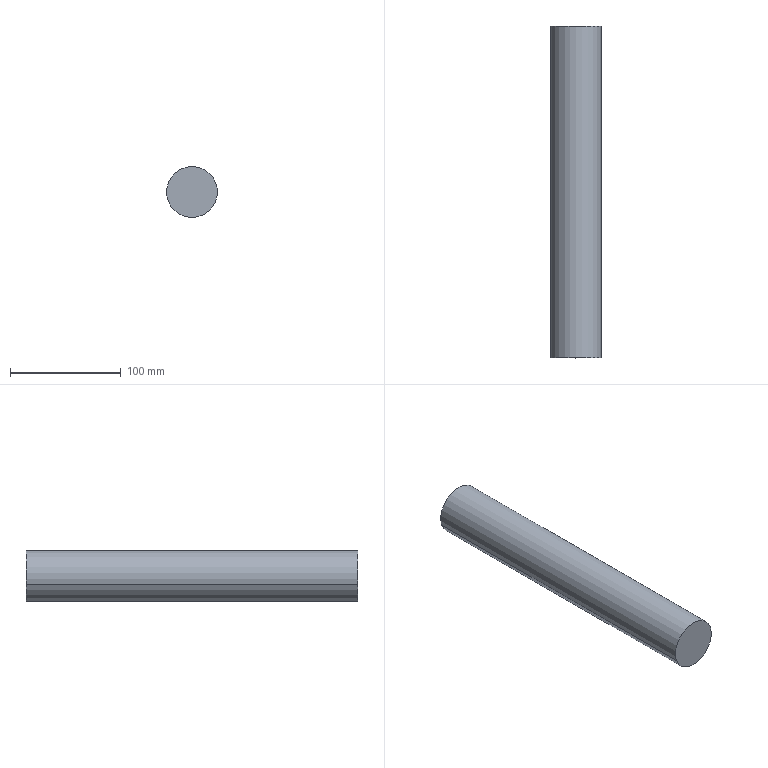Part | STEP file | Cylinder 1 | 1 solid | 4 faces | box 46 x 300 x 46 mm | volume 498571 mm3 | cylinder 2 | plane 2 | commonest cylinder face diameters 46 x2
STEP:
#1=CARTESIAN_POINT('',(-29.618,-109.099,478.073));
#2=VERTEX_POINT('',#1);
#3=CARTESIAN_POINT('',(-72.875,-109.099,462.427));
#4=VERTEX_POINT('',#3);
#5=CARTESIAN_POINT('',(-51.246,-109.099,470.25));
#6=DIRECTION('',(0.,-1.,0.));
#7=DIRECTION('',(0.9404,0.,0.3401));
#8=AXIS2_PLACEMENT_3D('',#5,#6,#7);
#9=CIRCLE('',#8,23.);
#10=EDGE_CURVE('',#2,#4,#9,.T.);
#11=ORIENTED_EDGE('',*,*,#10,.F.);
#12=CARTESIAN_POINT('',(-29.618,190.901,478.073));
#13=VERTEX_POINT('',#12);
#14=CARTESIAN_POINT('',(-29.618,-109.099,478.073));
#15=DIRECTION('',(0.,1.,0.));
#16=VECTOR('',#15,1000.);
#17=LINE('',#14,#16);
#18=EDGE_CURVE('',#2,#13,#17,.T.);
#19=ORIENTED_EDGE('',*,*,#18,.T.);
#20=CARTESIAN_POINT('',(-72.875,190.901,462.427));
#21=VERTEX_POINT('',#20);
#22=CARTESIAN_POINT('',(-51.246,190.901,470.25));
#23=DIRECTION('',(0.,-1.,0.));
#24=DIRECTION('',(0.9404,0.,0.3401));
#25=AXIS2_PLACEMENT_3D('',#22,#23,#24);
#26=CIRCLE('',#25,23.);
#27=EDGE_CURVE('',#13,#21,#26,.T.);
#28=ORIENTED_EDGE('',*,*,#27,.T.);
#29=CARTESIAN_POINT('',(-72.875,-109.099,462.427));
#30=DIRECTION('',(0.,1.,0.));
#31=VECTOR('',#30,1000.);
#32=LINE('',#29,#31);
#33=EDGE_CURVE('',#4,#21,#32,.T.);
#34=ORIENTED_EDGE('',*,*,#33,.F.);
#35=EDGE_LOOP('',(#11,#19,#28,#34));
#36=FACE_OUTER_BOUND('',#35,.T.);
#37=CARTESIAN_POINT('',(-51.246,-109.099,470.25));
#38=DIRECTION('',(0.,1.,0.));
#39=DIRECTION('',(-0.9404,0.,-0.3401));
#40=AXIS2_PLACEMENT_3D('',#37,#38,#39);
#41=CYLINDRICAL_SURFACE('',#40,23.);
#42=ADVANCED_FACE('',(#36),#41,.T.);
#43=CARTESIAN_POINT('',(-51.246,190.901,470.25));
#44=DIRECTION('',(0.,-1.,0.));
#45=DIRECTION('',(0.9404,0.,0.3401));
#46=AXIS2_PLACEMENT_3D('',#43,#44,#45);
#47=CIRCLE('',#46,23.);
#48=EDGE_CURVE('',#21,#13,#47,.T.);
#49=ORIENTED_EDGE('',*,*,#48,.F.);
#50=ORIENTED_EDGE('',*,*,#27,.F.);
#51=EDGE_LOOP('',(#49,#50));
#52=FACE_OUTER_BOUND('',#51,.T.);
#53=CARTESIAN_POINT('',(-51.246,190.901,470.25));
#54=DIRECTION('',(0.,-1.,0.));
#55=DIRECTION('',(0.9404,0.,0.3401));
#56=AXIS2_PLACEMENT_3D('',#53,#54,#55);
#57=PLANE('',#56);
#58=ADVANCED_FACE('',(#52),#57,.F.);
#59=CARTESIAN_POINT('',(-51.246,-109.099,470.25));
#60=DIRECTION('',(0.,-1.,0.));
#61=DIRECTION('',(0.9404,0.,0.3401));
#62=AXIS2_PLACEMENT_3D('',#59,#60,#61);
#63=CIRCLE('',#62,23.);
#64=EDGE_CURVE('',#4,#2,#63,.T.);
#65=ORIENTED_EDGE('',*,*,#64,.T.);
#66=ORIENTED_EDGE('',*,*,#10,.T.);
#67=EDGE_LOOP('',(#65,#66));
#68=FACE_OUTER_BOUND('',#67,.T.);
#69=CARTESIAN_POINT('',(-51.246,-109.099,470.25));
#70=DIRECTION('',(0.,-1.,0.));
#71=DIRECTION('',(0.9404,0.,0.3401));
#72=AXIS2_PLACEMENT_3D('',#69,#70,#71);
#73=PLANE('',#72);
#74=ADVANCED_FACE('',(#68),#73,.T.);
#75=ORIENTED_EDGE('',*,*,#18,.F.);
#76=ORIENTED_EDGE('',*,*,#64,.F.);
#77=ORIENTED_EDGE('',*,*,#33,.T.);
#78=ORIENTED_EDGE('',*,*,#48,.T.);
#79=EDGE_LOOP('',(#75,#76,#77,#78));
#80=FACE_OUTER_BOUND('',#79,.T.);
#81=CARTESIAN_POINT('',(-51.246,-109.099,470.25));
#82=DIRECTION('',(0.,1.,0.));
#83=DIRECTION('',(-0.9404,0.,-0.3401));
#84=AXIS2_PLACEMENT_3D('',#81,#82,#83);
#85=CYLINDRICAL_SURFACE('',#84,23.);
#86=ADVANCED_FACE('',(#80),#85,.T.);
#87=CLOSED_SHELL('',(#42,#58,#74,#86));
#88=MANIFOLD_SOLID_BREP('',#87);
#89=CARTESIAN_POINT('',(0.,0.,0.));
#90=DIRECTION('',(0.,0.,1.));
#91=DIRECTION('',(1.,0.,0.));
#92=AXIS2_PLACEMENT_3D('',#89,#90,#91);
#93=(LENGTH_UNIT()NAMED_UNIT(*)SI_UNIT(.MILLI.,.METRE.));
#94=UNCERTAINTY_MEASURE_WITH_UNIT(LENGTH_MEASURE(0.00001),#93,'','');
#95=(NAMED_UNIT(*)PLANE_ANGLE_UNIT()SI_UNIT($,.RADIAN.));
#96=(NAMED_UNIT(*)SI_UNIT($,.STERADIAN.)SOLID_ANGLE_UNIT());
#97=(GEOMETRIC_REPRESENTATION_CONTEXT(3)GLOBAL_UNCERTAINTY_ASSIGNED_CONTEXT((#94))GLOBAL_UNIT_ASSIGNED_CONTEXT((#93,#95,#96))REPRESENTATION_CONTEXT('',''));
#98=ADVANCED_BREP_SHAPE_REPRESENTATION('',(#88,#92),#97);